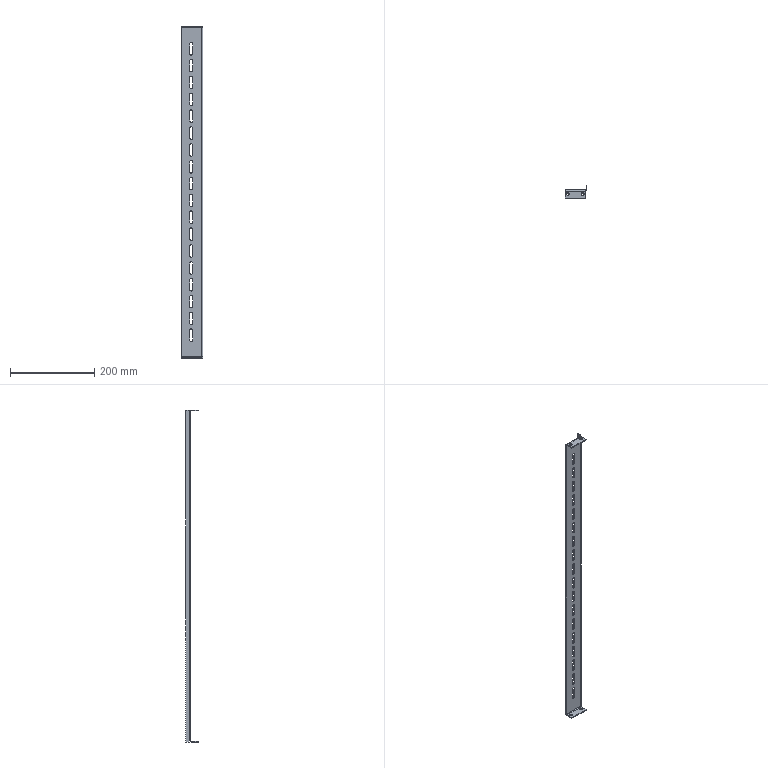Part | STEP file | 1 solid | 130 faces | box 52 x 30 x 788 mm | volume 91760 mm3 | cylinder 68 | plane 62 | commonest cylinder face diameters 7 x65 3 x3